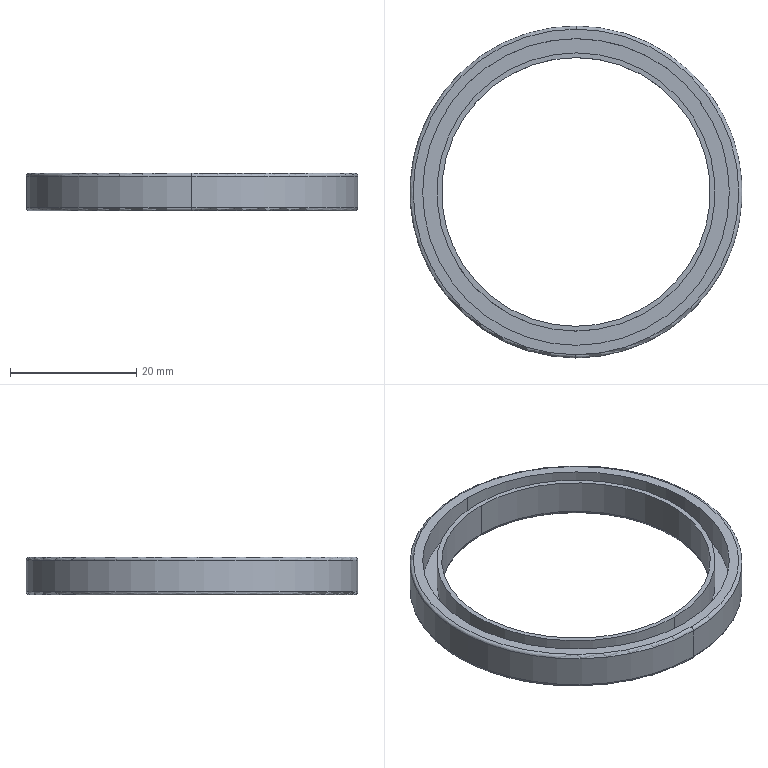Part | STEP file | 2026.6.15-Main Assembly图.sldasm-Part-118 | 1 solid | 98 faces | box 52.5 x 52.5 x 6 mm | volume 2953 mm3 | plane 84 | cylinder 8 | torus 6 | commonest cylinder face diameters 42.5 x2 44 x2 48.5 x2 52.5 x2